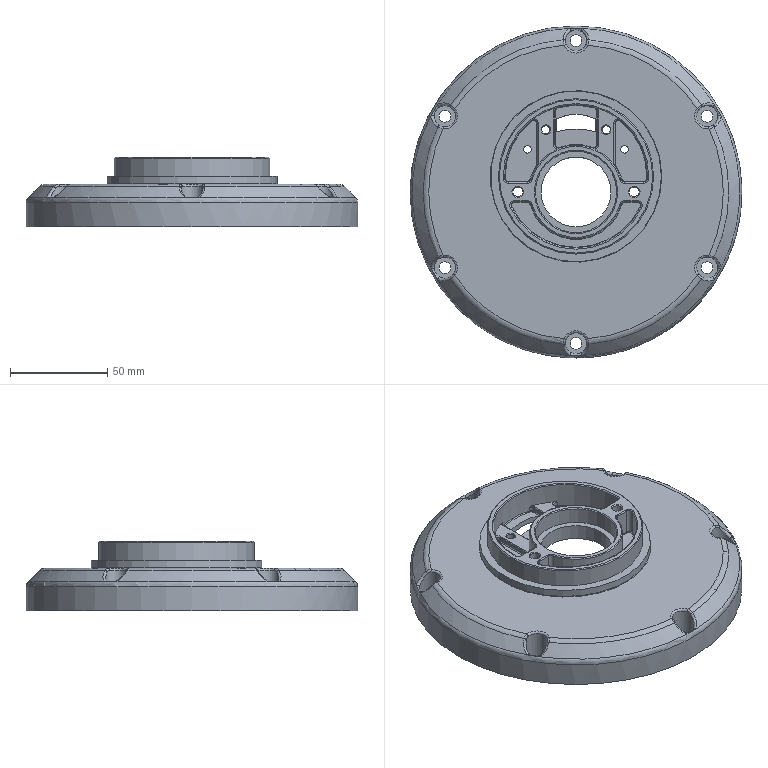NC program | NX | posted with a generic post | part box 171 x 171 x 36 mm
Lines 8896 to 9772 of 127321:
(3D开粗 , TOOL : D6-L25)
N17790 T06 M6
N17792 G54
N17794 G17 G0 G90 X-5.475 Y81.132 S4500 M3
N17796 G43 Z20. H6
N17798 Z-13.83
N17800 G94 G1 Z-14.13 F2500.
N17802 G3 X-4.846 Y79.67 R1.2
N17804 G2 X-3.558 Y78.677 R3.759
N17806 X-2.56 Y76.984 R6.052
N17808 G3 X2.56 Y76.984 R2.755
N17810 G2 X3.545 Y78.661 R6.058
N17812 X4.867 Y79.678 R3.774
N17814 G3 X5.505 Y81.136 R1.2
N17816 G1 Z-13.83
N17818 X-6.033 Y81.749 Z-14.08 F15000.
N17820 Z-14.38 F2500.
N17822 G3 X-5.25 Y80.358 R1.2
N17824 G2 X-3.233 Y78.81 R3.992
N17826 X-2.349 Y77.068 R8.343
N17828 G3 X2.349 Y77.068 R2.527
N17830 G2 X2.709 Y77.901 R96.005
N17832 X4.066 Y79.708 R5.064
N17834 X5.192 Y80.36 R3.692
N17836 G3 X5.953 Y81.755 R1.2
N17838 G1 Z-14.08
N17840 X-6.228 Y82.168 Z-14.33 F15000.
N17842 Z-14.63 F2500.
N17844 G3 X-5.392 Y80.809 R1.2
N17846 G2 X-3.291 Y79.303 R3.983
N17848 G1 X-3.202 Y79.172
N17850 X-2.971 Y78.81
N17852 X-2.955 Y78.782
N17854 X-2.709 Y78.304
N17856 X-2.453 Y77.677
N17858 X-2.437 Y77.624
N17860 X-2.421 Y77.585
N17862 X-2.233 Y77.114
N17864 G3 X2.233 Y77.114 R2.403
N17866 G2 X2.668 Y78.201 R59.523
N17868 X3.714 Y79.793 R5.013
N17870 X5.386 Y80.81 R3.922
N17872 G3 X6.219 Y82.17 R1.2
N17874 G1 Z-14.33
N17876 X-6.346 Y82.495 Z-14.58 F15000.
N17878 Z-14.88 F2500.
N17880 G3 X-5.479 Y81.154 R1.2
N17882 G2 X-3.418 Y79.795 R3.998
N17884 X-2.463 Y77.975 R5.637
N17886 G3 X-2.181 Y77.134 R14.719
N17888 X2.181 Y77.134 R2.346
N17890 G1 X2.232 Y77.263
N17892 X2.463 Y77.973
N17894 G2 X3.418 Y79.795 R5.626
N17896 X5.471 Y81.155 R3.976
N17898 G3 X6.337 Y82.495 R1.2
N17900 G1 Z-14.58
N17902 X-6.409 Y82.764 Z-14.83 F15000.
N17904 Z-15.13 F2500.
N17906 G3 X-5.523 Y81.436 R1.2
N17908 G2 X-3.448 Y80.112 R3.995
N17910 X-2.501 Y78.317 R5.042
N17912 X-2.279 Y77.47 R10.733
N17914 G3 X2.283 Y77.488 R2.34
N17916 G2 X2.677 Y78.81 R8.545
N17918 X3.694 Y80.378 R4.631
N17920 X5.522 Y81.437 R3.974
N17922 G3 X6.407 Y82.765 R1.2
N17924 G1 Z-14.83
N17926 X-6.412 Y83.016 Z-15.08 F15000.
N17928 Z-15.38 F2500.
N17930 G3 X-5.524 Y81.69 R1.2
N17932 G2 X-3.448 Y80.365 R3.982
N17934 G1 X-3.39 Y80.288
N17936 X-3.202 Y80.04
N17938 G2 X-2.362 Y77.947 R5.292
N17940 G1 X-2.344 Y77.825
N17942 X-2.315 Y77.657
N17944 X-2.29 Y77.519
N17946 X-2.279 Y77.47
N17948 G3 X2.283 Y77.488 R2.34
N17950 G1 X2.293 Y77.532
N17952 X2.314 Y77.653
N17954 G2 X2.782 Y79.303 R5.856
N17956 X4.433 Y81.22 R4.368
N17958 X5.516 Y81.69 R3.887
N17960 G3 X6.398 Y83.017 R1.2
N17962 G1 Z-15.08
N17964 X-6.398 Y83.268 Z-15.33 F15000.
N17966 Z-15.63 F2500.
N17968 G3 X-5.513 Y81.941 R1.2
N17970 G2 X-3.694 Y80.884 R3.937
N17972 X-2.436 Y78.463 R4.779
N17974 X-2.33 Y77.788 R4.589
N17976 G3 X-2.29 Y77.519 R2.34
N17978 G1 X-2.279 Y77.47
N17980 G3 X2.283 Y77.488 R2.34
N17982 G1 X2.293 Y77.532
N17984 X2.314 Y77.653
N17986 X2.323 Y77.718
N17988 X2.33 Y77.788
N17990 G2 X2.906 Y79.795 R5.32
N17992 G1 X2.955 Y79.899
N17994 G2 X4.926 Y81.736 R4.272
N17996 X5.495 Y81.942 R3.708
N17998 G3 X6.366 Y83.272 R1.2
N18000 G1 Z-15.33
N18002 X-6.384 Y83.52 Z-15.58 F15000.
N18004 Z-15.88 F2500.
N18006 G3 X-5.501 Y82.193 R1.2
N18008 G2 X-3.694 Y81.144 R3.924
N18010 X-2.6 Y79.303 R4.475
N18012 X-2.337 Y77.89 R5.004
N18014 G1 X-2.333 Y77.82
N18016 X-2.33 Y77.788
N18018 G3 X-2.29 Y77.519 R2.34
N18020 G1 X-2.279 Y77.47
N18022 G3 X2.283 Y77.488 R2.34
N18024 G1 X2.293 Y77.532
N18026 X2.314 Y77.653
N18028 X2.323 Y77.718
N18030 X2.337 Y77.89
N18032 G2 X2.784 Y79.795 R5.282
N18034 G1 X2.955 Y80.157
N18036 X3.154 Y80.471
N18038 G2 X4.636 Y81.842 R3.941
N18040 G1 X4.716 Y81.884
N18042 G2 X5.497 Y82.193 R3.764
N18044 G3 X6.372 Y83.522 R1.2
N18046 G1 Z-15.58
N18048 X-6.344 Y83.774 Z-15.83 F15000.
N18050 Z-16.13 F2500.
N18052 G3 X-5.466 Y82.446 R1.2
N18054 G2 X-4.11 Y81.775 R3.835
N18056 X-2.671 Y79.795 R4.362
N18058 X-2.34 Y77.98 R5.395
N18060 G1 X-2.333 Y77.82
N18062 X-2.33 Y77.788
N18064 X-2.322 Y77.711
N18066 X-2.29 Y77.519
N18068 X-2.279 Y77.47
N18070 G3 X2.283 Y77.488 R2.34
N18072 G1 X2.293 Y77.532
N18074 X2.314 Y77.653
N18076 X2.323 Y77.718
N18078 G3 X2.34 Y77.98 R2.34
N18080 G2 X2.73 Y79.95 R5.395
N18082 X4.05 Y81.729 R4.377
N18084 X5.466 Y82.446 R3.844
N18086 G3 X6.345 Y83.774 R1.2
N18088 G1 Z-15.83
N18090 X-6.319 Y84.026 Z-16.08 F15000.
N18092 Z-16.38 F2500.
N18094 G3 X-5.438 Y82.697 R1.2
N18096 G2 X-3.202 Y81.118 R3.928
N18098 G1 X-2.993 Y80.78
N18100 X-2.955 Y80.721
N18102 X-2.745 Y80.288
N18104 X-2.709 Y80.206
N18106 X-2.607 Y79.904
N18108 G2 X-2.336 Y78.317 R5.125
N18110 G1 X-2.343 Y78.253
N18112 X-2.339 Y78.163
N18114 Y78.071
N18116 G3 X-2.333 Y77.82 R2.34
N18118 G1 X-2.33 Y77.788
N18120 X-2.321 Y77.705
N18122 X-2.29 Y77.519
N18124 X-2.279 Y77.47
N18126 G3 X2.283 Y77.488 R2.34
N18128 G1 X2.293 Y77.532
N18130 X2.314 Y77.653
N18132 X2.323 Y77.718
N18134 G3 X2.339 Y78.071 R2.34
N18136 G2 X2.441 Y79.303 R5.682
N18138 X3.448 Y81.439 R4.76
N18140 X5.432 Y82.697 R3.907
N18142 G3 X6.312 Y84.026 R1.2
N18144 G1 Z-16.08
N18146 X-6.256 Y84.282 Z-16.33 F15000.
N18148 Z-16.63 F2500.
N18150 G3 X-5.379 Y82.952 R1.2
N18152 G2 X-3.384 Y81.659 R3.854
N18154 X-2.416 Y79.549 R4.658
N18156 X-2.334 Y78.162 R5.651
N18158 G3 X-2.337 Y77.89 R2.34
N18160 G1 X-2.333 Y77.82
N18162 X-2.33 Y77.788
N18164 G3 X-2.29 Y77.519 R2.34
N18166 G1 X-2.279 Y77.47
N18168 G3 X2.266 Y77.416 R2.34
N18170 G1 X2.283 Y77.488
N18172 X2.293 Y77.532
N18174 X2.314 Y77.653
N18176 X2.325 Y77.738
N18178 X2.333 Y77.818
N18180 X2.338 Y77.899
N18182 G3 X2.335 Y78.152 R2.34
N18184 G2 X2.69 Y80.49 R5.29
N18186 X3.943 Y82.211 R4.254
N18188 X5.38 Y82.952 R3.828
N18190 G3 X6.255 Y84.282 R1.2
N18192 G1 Z-16.33
N18194 X-6.245 Y84.533 Z-16.58 F15000.
N18196 Z-16.88 F2500.
N18198 G3 X-5.36 Y83.206 R1.2
N18200 G2 X-2.955 Y81.373 R3.925
N18202 X-2.299 Y79.042 R4.937
N18204 X-2.326 Y78.253 R5.852
N18206 G3 X-2.333 Y77.82 R2.34
N18208 G1 X-2.33 Y77.788
N18210 G3 X-2.29 Y77.519 R2.34
N18212 G1 X-2.279 Y77.47
N18214 X-2.272 Y77.44
N18216 G3 X2.283 Y77.488 R2.34
N18218 G1 X2.293 Y77.532
N18220 X2.314 Y77.653
N18222 X2.325 Y77.738
N18224 X2.335 Y77.843
N18226 G3 X2.335 Y78.152 R2.34
N18228 G1 X2.333 Y78.183
N18230 X2.325 Y78.264
N18232 G2 X2.709 Y80.902 R5.234
N18234 X4.433 Y82.841 R4.181
N18236 X5.335 Y83.208 R3.847
N18238 G3 X6.216 Y84.535 R1.2
N18240 G1 Z-16.58
N18242 X-6.158 Y84.791 Z-16.83 F15000.
N18244 Z-17.13 F2500.
N18246 G3 X-5.279 Y83.46 R1.2
N18248 G2 X-2.706 Y81.273 R3.924
N18250 X-2.294 Y78.532 R5.128
N18252 G1 X-2.314 Y78.345
N18254 G3 X-2.336 Y77.867 R2.34
N18256 G1 X-2.333 Y77.82
N18258 X-2.33 Y77.788
N18260 G3 X-2.29 Y77.519 R2.34
N18262 G1 X-2.278 Y77.463
N18264 G3 X2.283 Y77.488 R2.34
N18266 G1 X2.293 Y77.532
N18268 X2.314 Y77.653
N18270 X2.323 Y77.718
N18272 G3 X2.335 Y78.152 R2.34
N18274 G1 X2.333 Y78.183
N18276 X2.314 Y78.345
N18278 G2 X2.51 Y80.78 R5.325
N18280 X4.926 Y83.358 R4.062
N18282 X5.24 Y83.463 R3.593
N18284 G3 X6.1 Y84.797 R1.2
N18286 G1 Z-16.83
N18288 X-6.065 Y85.047 Z-17.08 F15000.
N18290 Z-17.38 F2500.
N18292 G3 X-5.189 Y83.715 R1.2
N18294 G2 X-2.528 Y81.273 R3.915
N18296 X-2.271 Y78.624 R5.144
N18298 G1 X-2.318 Y78.317
N18300 G3 X-2.337 Y77.89 R2.34
N18302 G1 X-2.333 Y77.82
N18304 X-2.33 Y77.788
N18306 G3 X-2.29 Y77.519 R2.34
N18308 G1 X-2.279 Y77.47
N18310 G3 X2.283 Y77.488 R2.34
N18312 G1 X2.293 Y77.532
N18314 X2.314 Y77.653
N18316 X2.323 Y77.718
N18318 X2.338 Y77.899
N18320 G3 X2.335 Y78.152 R2.34
N18322 G1 X2.333 Y78.183
N18324 G3 X2.299 Y78.436 R2.34
N18326 G2 X2.264 Y80.288 R5.517
N18328 X3.065 Y82.258 R4.438
N18330 X5.17 Y83.716 R3.843
N18332 G3 X6.042 Y85.049 R1.2
N18334 G1 Z-17.08
N18336 X-5.966 Y85.306 Z-17.33 F15000.
N18338 Z-17.63 F2500.
N18340 G3 X-5.092 Y83.973 R1.2
N18342 G2 X-2.542 Y81.765 R3.882
N18344 X-2.207 Y78.915 R5.025
N18346 G1 X-2.279 Y78.529
N18348 X-2.307 Y78.393
N18350 X-2.318 Y78.317
N18352 G3 X-2.337 Y77.89 R2.34
N18354 G1 X-2.333 Y77.82
N18356 X-2.33 Y77.788
N18358 G3 X-2.29 Y77.519 R2.34
N18360 G1 X-2.279 Y77.47
N18362 G3 X2.283 Y77.488 R2.34
N18364 G1 X2.293 Y77.532
N18366 X2.301 Y77.575
N18368 X2.314 Y77.653
N18370 X2.323 Y77.718
N18372 X2.327 Y77.75
N18374 X2.338 Y77.899
N18376 G3 X2.335 Y78.152 R2.34
N18378 G1 X2.333 Y78.183
N18380 G3 X2.28 Y78.529 R2.34
N18382 G2 X2.229 Y80.78 R5.431
N18384 X3.448 Y83.057 R4.27
N18386 X5.047 Y83.976 R3.724
N18388 G3 X5.912 Y85.311 R1.2
N18390 G1 Z-17.33
N18392 X-5.828 Y85.566 Z-17.58 F15000.
N18394 Z-17.88 F2500.
N18396 G3 X-4.961 Y84.231 R1.2
N18398 G2 X-2.861 Y82.75 R3.807
N18400 X-2.089 Y80.65 R4.204
N18402 G1 X-2.078 Y80.514
N18404 G2 X-2.255 Y78.623 R5.42
N18406 G3 X-2.307 Y78.393 R2.34
N18408 G1 X-2.318 Y78.317
N18410 G3 X-2.337 Y77.89 R2.34
N18412 G1 X-2.333 Y77.82
N18414 X-2.33 Y77.788
N18416 G3 X-2.29 Y77.519 R2.34
N18418 G1 X-2.279 Y77.47
N18420 G3 X2.283 Y77.488 R2.34
N18422 G1 X2.293 Y77.532
N18424 X2.314 Y77.653
N18426 X2.323 Y77.718
N18428 G3 X2.335 Y78.152 R2.34
N18430 G1 X2.333 Y78.183
N18432 G3 X2.256 Y78.621 R2.34
N18434 G2 X2.217 Y81.383 R5.381
N18436 X3.94 Y83.781 R4.077
N18438 X4.932 Y84.232 R3.652
N18440 G3 X5.79 Y85.57 R1.2
N18442 G1 Z-17.58
N18444 X-5.729 Y85.823 Z-17.83 F15000.
N18446 Z-18.13 F2500.
N18448 G3 X-4.86 Y84.487 R1.2
N18450 G2 X-2.145 Y81.765 R3.876
N18452 G1 X-2.03 Y81.273
N18454 G2 X-2.134 Y79.045 R5.404
N18456 G1 X-2.179 Y78.904
N18458 X-2.229 Y78.713
N18460 G3 X-2.307 Y78.393 R2.34
N18462 G1 X-2.318 Y78.317
N18464 G3 X-2.337 Y77.89 R2.34
N18466 G1 X-2.333 Y77.82
N18468 X-2.33 Y77.788
N18470 G3 X-2.29 Y77.519 R2.34
N18472 G1 X-2.279 Y77.47
N18474 G3 X2.283 Y77.488 R2.34
N18476 G1 X2.293 Y77.532
N18478 X2.314 Y77.653
N18480 X2.323 Y77.718
N18482 G3 X2.335 Y78.152 R2.34
N18484 G1 X2.333 Y78.183
N18486 G3 X2.232 Y78.703 R2.34
N18488 G2 X2.03 Y81.273 R5.484
N18490 X3.448 Y83.767 R4.13
N18492 X4.837 Y84.489 R3.803
N18494 G3 X5.702 Y85.825 R1.2
N18496 G1 Z-17.83
N18498 X-5.583 Y86.084 Z-18.08 F15000.
N18500 Z-18.38 F2500.
N18502 G3 X-4.716 Y84.747 R1.2
N18504 G2 X-1.97 Y81.824 R3.857
N18506 X-2.132 Y78.996 R5.26
N18508 G1 X-2.134 Y78.985
N18510 X-2.167 Y78.9
N18512 X-2.197 Y78.805
N18514 G3 X-2.307 Y78.393 R2.34
N18516 G1 X-2.318 Y78.317
N18518 G3 X-2.333 Y77.82 R2.34
N18520 G1 X-2.33 Y77.788
N18522 G3 X-2.29 Y77.519 R2.34
N18524 G1 X-2.279 Y77.47
N18526 G3 X2.283 Y77.488 R2.34
N18528 G1 X2.293 Y77.532
N18530 X2.314 Y77.653
N18532 X2.323 Y77.718
N18534 G3 X2.335 Y78.152 R2.34
N18536 G1 X2.333 Y78.183
N18538 G3 X2.232 Y78.703 R2.34
N18540 G1 X2.221 Y78.736
N18542 X2.197 Y78.805
N18544 G2 X1.874 Y81.273 R5.553
N18546 X2.955 Y83.697 R4.229
N18548 X4.703 Y84.748 R3.826
N18550 G3 X5.567 Y86.085 R1.2
N18552 G1 Z-18.08
N18554 X-5.412 Y86.345 Z-18.33 F15000.
N18556 Z-18.63 F2500.
N18558 G3 X-4.55 Y85.006 R1.2
N18560 G2 X-1.869 Y82.258 R3.832
N18562 G1 X-1.77 Y81.765
N18564 G2 X-2.049 Y79.19 R5.302
N18566 G1 X-2.091 Y79.092
N18568 X-2.161 Y78.898
N18570 G3 X-2.307 Y78.393 R2.34
N18572 G1 X-2.318 Y78.317
N18574 G3 X-2.337 Y77.89 R2.34
N18576 G1 X-2.333 Y77.82
N18578 X-2.33 Y77.788
N18580 G3 X-2.29 Y77.519 R2.34
N18582 G1 X-2.279 Y77.47
N18584 G3 X2.283 Y77.488 R2.34
N18586 G1 X2.293 Y77.532
N18588 X2.314 Y77.653
N18590 X2.323 Y77.718
N18592 G3 X2.335 Y78.152 R2.34
N18594 G1 X2.333 Y78.183
N18596 G3 X2.251 Y78.638 R2.34
N18598 G1 X2.232 Y78.703
N18600 X2.221 Y78.736
N18602 X2.191 Y78.82
N18604 X2.161 Y78.898
N18606 G2 X1.87 Y79.795 R6.981
N18608 X1.97 Y82.579 R4.89
N18610 X4.545 Y85.006 R3.817
N18612 G3 X5.406 Y86.346 R1.2
N18614 G1 Z-18.33
N18616 X-5.233 Y86.607 Z-18.58 F15000.
N18618 Z-18.88 F2500.
N18620 G3 X-4.374 Y85.266 R1.2
N18622 G2 X-1.649 Y82.258 R3.826
N18624 X-1.97 Y79.339 R5.327
N18626 G1 X-1.985 Y79.303
N18628 X-2.039 Y79.186
N18630 X-2.134 Y78.959
N18632 G3 X-2.307 Y78.393 R2.34
N18634 G1 X-2.318 Y78.317
N18636 G3 X-2.333 Y77.82 R2.34
N18638 G1 X-2.33 Y77.788
N18640 G3 X-2.29 Y77.518 R2.34
N18642 G1 X-2.279 Y77.47
N18644 G3 X2.283 Y77.488 R2.34
N18646 G1 X2.293 Y77.532
N18648 X2.314 Y77.653
N18650 X2.323 Y77.718
N18652 X2.333 Y77.816
N18654 G3 X2.335 Y78.152 R2.34
N18656 G1 X2.333 Y78.183
N18658 G3 X2.232 Y78.703 R2.34
N18660 G1 X2.221 Y78.736
N18662 G3 X2.12 Y78.991 R2.34
N18664 G2 X1.809 Y79.795 R8.055
N18666 X1.648 Y82.258 R5.191
N18668 X4.373 Y85.266 R3.825
N18670 G3 X5.232 Y86.607 R1.2
N18672 G1 Z-18.58
N18674 X-5.009 Y86.87 Z-18.83 F15000.
N18676 Z-19.13 F2500.
N18678 G3 X-4.158 Y85.525 R1.2
N18680 G2 X-1.477 Y82.527 R3.788
N18682 X-1.609 Y80.242 R5.076
N18684 X-2.085 Y79.062 R6.477
N18686 G3 X-2.307 Y78.393 R2.34
N18688 G1 X-2.318 Y78.317
N18690 G3 X-2.337 Y77.89 R2.34
N18692 G1 X-2.333 Y77.82
N18694 X-2.33 Y77.788
N18696 G3 X-2.29 Y77.518 R2.34
N18698 G1 X-2.279 Y77.47
N18700 G3 X2.283 Y77.488 R2.34
N18702 G1 X2.293 Y77.532
N18704 X2.314 Y77.653
N18706 X2.323 Y77.722
N18708 G3 X2.335 Y78.152 R2.34
N18710 G1 X2.333 Y78.183
N18712 G3 X2.232 Y78.703 R2.34
N18714 G1 X2.221 Y78.738
N18716 X2.191 Y78.82
N18718 G3 X2.074 Y79.084 R2.34
N18720 G2 X1.597 Y80.288 R6.965
N18722 X1.522 Y82.75 R4.849
N18724 X4.156 Y85.525 R3.787
N18726 G3 X5.007 Y86.87 R1.2
N18728 G1 Z-18.83
N18730 X-4.792 Y87.133 Z-19.08 F15000.
N18732 Z-19.38 F2500.
N18734 G3 X-3.943 Y85.786 R1.2
N18736 G2 X-1.21 Y82.258 R3.796
N18738 X-1.735 Y79.728 R5.463
N18740 X-2.022 Y79.178 R8.409
N18742 G1 X-2.068 Y79.095
N18744 X-2.085 Y79.062
N18746 G3 X-2.307 Y78.393 R2.34
N18748 G1 X-2.318 Y78.317
N18750 G3 X-2.336 Y77.867 R2.34
N18752 G1 X-2.333 Y77.82
N18754 X-2.33 Y77.788
N18756 G3 X-2.29 Y77.518 R2.34
N18758 G1 X-2.279 Y77.47
N18760 G3 X2.283 Y77.488 R2.34
N18762 G1 X2.293 Y77.532
N18764 X2.314 Y77.653
N18766 X2.323 Y77.722
N18768 X2.333 Y77.816
N18770 X2.338 Y77.899
N18772 G3 X2.335 Y78.152 R2.34
N18774 G1 X2.331 Y78.204
N18776 X2.313 Y78.356
N18778 X2.299 Y78.437
N18780 X2.277 Y78.54
N18782 X2.251 Y78.638
N18784 X2.232 Y78.703
N18786 X2.221 Y78.738
N18788 X2.191 Y78.82
N18790 X2.133 Y78.962
N18792 X2.12 Y78.991
N18794 G3 X2.022 Y79.178 R2.34
N18796 G2 X1.22 Y81.611 R5.957
N18798 X2.214 Y84.721 R4.085
N18800 X3.944 Y85.786 R3.814
N18802 G3 X4.793 Y87.133 R1.2
N18804 G1 Z-19.08
N18806 X-4.529 Y87.398 Z-19.33 F15000.
N18808 Z-19.63 F2500.
N18810 G3 X-3.686 Y86.048 R1.2
N18812 G2 X-0.985 Y82.515 R3.773
N18814 X-1.423 Y80.291 R5.27
N18816 X-1.964 Y79.273 R7.469
N18818 G3 X-2.068 Y79.095 R2.34
N18820 G1 X-2.085 Y79.062
N18822 G3 X-2.307 Y78.393 R2.34
N18824 G1 X-2.318 Y78.317
N18826 G3 X-2.337 Y77.89 R2.34
N18828 G1 X-2.333 Y77.82
N18830 X-2.33 Y77.788
N18832 G3 X-2.29 Y77.518 R2.34
N18834 G1 X-2.279 Y77.47
N18836 G3 X2.283 Y77.488 R2.34
N18838 G1 X2.293 Y77.532
N18840 X2.314 Y77.653
N18842 X2.323 Y77.718
N18844 X2.333 Y77.816
N18846 X2.338 Y77.899
N18848 G3 X2.335 Y78.152 R2.34
N18850 G1 X2.333 Y78.183
N18852 G3 X2.277 Y78.54 R2.34
N18854 G1 X2.251 Y78.638
N18856 X2.232 Y78.703
N18858 X2.221 Y78.736
N18860 X2.191 Y78.82
N18862 G3 X1.964 Y79.272 R2.34
N18864 G2 X1.325 Y80.534 R7.072
N18866 X0.985 Y82.549 R5.201
N18868 X3.682 Y86.048 R3.771
N18870 G3 X4.524 Y87.398 R1.2
N18872 G1 Z-19.33
N18874 X-4.251 Y87.662 Z-19.58 F15000.
N18876 Z-19.88 F2500.
N18878 G3 X-3.413 Y86.31 R1.2
N18880 G2 X-0.749 Y82.258 R3.772
N18882 G1 X-0.82 Y81.765
N18884 G2 X-1.806 Y79.506 R6.112
N18886 G1 X-1.835 Y79.469
N18888 X-1.899 Y79.367
N18890 G3 X-2.068 Y79.095 R2.34
N18892 G1 X-2.085 Y79.062
N18894 G3 X-2.307 Y78.393 R2.34
N18896 G1 X-2.318 Y78.317
N18898 G3 X-2.337 Y77.89 R2.34
N18900 G1 X-2.333 Y77.82
N18902 X-2.33 Y77.788
N18904 G3 X-2.29 Y77.518 R2.34
N18906 G1 X-2.279 Y77.47
N18908 G3 X2.275 Y77.453 R2.34
N18910 G1 X2.283 Y77.488
N18912 X2.293 Y77.532
N18914 X2.314 Y77.653
N18916 X2.325 Y77.734
N18918 X2.338 Y77.899
N18920 G3 X2.335 Y78.152 R2.34
N18922 G1 X2.333 Y78.183
N18924 G3 X2.277 Y78.54 R2.34
N18926 G1 X2.251 Y78.638
N18928 X2.232 Y78.703
N18930 X2.221 Y78.736
N18932 X2.191 Y78.82
N18934 G3 X1.899 Y79.367 R2.34
N18936 G2 X1.22 Y80.534 R7.37
N18938 X0.719 Y82.75 R5.392
N18940 X3.41 Y86.31 R3.775
N18942 G3 X4.249 Y87.662 R1.2
N18944 G1 Z-19.58
N18946 X-3.943 Y87.926 Z-19.83 F15000.
N18948 Z-20.13 F2500.
N18950 G3 X-3.107 Y86.571 R1.2
N18952 G2 X-0.84 Y84.721 R3.83
N18954 X-0.64 Y81.639 R4.134
N18956 X-1.827 Y79.462 R6.884
N18958 G3 X-2.068 Y79.095 R2.34
N18960 G1 X-2.085 Y79.062
N18962 G3 X-2.307 Y78.393 R2.34
N18964 G1 X-2.318 Y78.317
N18966 G3 X-2.333 Y77.82 R2.34
N18968 G1 X-2.33 Y77.788
N18970 G3 X-2.29 Y77.518 R2.34
N18972 G1 X-2.279 Y77.47
N18974 G3 X2.283 Y77.488 R2.34
N18976 G1 X2.293 Y77.532
N18978 X2.314 Y77.653
N18980 X2.323 Y77.718
N18982 G3 X2.335 Y78.152 R2.34
N18984 G1 X2.333 Y78.183
N18986 G3 X2.232 Y78.704 R2.34
N18988 G1 X2.221 Y78.736
N18990 G3 X1.827 Y79.462 R2.34
N18992 G2 X0.638 Y81.642 R6.843
N18994 X0.839 Y84.721 R4.137
N18996 X3.106 Y86.571 R3.829
N18998 G3 X3.942 Y87.926 R1.2
N19000 G1 Z-19.83
N19002 X-3.593 Y88.19 Z-20.08 F15000.
N19004 Z-20.38 F2500.
N19006 G3 X-2.75 Y86.833 R1.2
N19008 G2 X-1.478 Y86.199 R4.062
N19010 X-0.268 Y82.063 R3.771
N19012 X-1.301 Y80.11 R6.821
N19014 G1 X-1.478 Y79.876
N19016 X-1.543 Y79.795
N19018 X-1.57 Y79.763
N19020 X-1.642 Y79.684
N19022 X-1.664 Y79.66
N19024 X-1.746 Y79.557
N19026 G3 X-2.068 Y79.095 R2.34
N19028 G1 X-2.085 Y79.062
N19030 G3 X-2.307 Y78.393 R2.34
N19032 G1 X-2.318 Y78.317
N19034 G3 X-2.333 Y77.82 R2.34
N19036 G1 X-2.33 Y77.788
N19038 G3 X-2.29 Y77.518 R2.34
N19040 G1 X-2.279 Y77.47
N19042 G3 X2.283 Y77.488 R2.34
N19044 G1 X2.293 Y77.532
N19046 X2.314 Y77.653
N19048 X2.323 Y77.718
N19050 X2.333 Y77.816
N19052 X2.338 Y77.899
N19054 G3 X2.335 Y78.152 R2.34
N19056 G1 X2.333 Y78.183
N19058 G3 X2.277 Y78.54 R2.34
N19060 G1 X2.251 Y78.638
N19062 X2.232 Y78.704
N19064 X2.221 Y78.736
N19066 X2.191 Y78.82
N19068 G3 X1.747 Y79.557 R2.34
N19070 G2 X0.436 Y81.602 R7.492
N19072 X0.101 Y83.67 R4.298
N19074 X2.713 Y86.834 R3.608
N19076 G3 X3.572 Y88.17 R1.2
N19078 G1 Z-20.08
N19080 X-3.119 Y88.452 Z-20.33 F15000.
N19082 Z-20.63 F2500.
N19084 G3 X-2.24 Y87.099 R1.2
N19086 G2 X-1.191 Y86.691 R5.01
N19088 X0. Y85.461 R2.735
N19090 X1.97 Y87.031 R3.381
N19092 X2.23 Y87.099 R6.01
N19094 G3 X3.14 Y88.445 R1.2
N19096 G1 Z-20.33
N19098 G0 Z20.
N19100 X-2.13 Y77.375
N19102 Z-19.38
N19104 G3 X-2.13 Y77.375 Z-19.88 I2.188 J0.641
N19106 X-2.13 Y77.375 Z-20.381 I2.188 J0.641
N19108 X2.251 Y78.639 Z-20.63 R2.28
N19110 G1 X2.248 Y78.65
N19112 X2.245 Y78.659
N19114 X2.232 Y78.704
N19116 X2.221 Y78.736
N19118 G3 X1.657 Y79.652 R2.34
N19120 G2 X0.384 Y81.273 R8.531
N19122 X0. Y82.034 R5.24
N19124 X-1.296 Y80.041 R7.204
N19126 G1 X-1.657 Y79.653
N19128 G3 X-2.068 Y79.095 R2.34
N19130 G1 X-2.085 Y79.062
N19132 G3 X-2.307 Y78.393 R2.34
N19134 G1 X-2.318 Y78.317
N19136 G3 X-2.333 Y77.82 R2.34
N19138 G1 X-2.33 Y77.788
N19140 G3 X-2.301 Y77.576 R2.34
N19142 G1 X-2.271 Y77.434
N19144 G3 X2.283 Y77.488 R2.34
N19146 G1 X2.294 Y77.54
N19148 X2.3 Y77.582
N19150 X2.304 Y77.592
N19152 X2.314 Y77.653
N19154 X2.323 Y77.718
N19156 G3 X2.335 Y78.152 R2.34
N19158 G1 X2.333 Y78.183
N19160 G3 X2.248 Y78.65 R2.34
N19162 G1 X2.245 Y78.659
N19164 X2.232 Y78.704
N19166 X2.221 Y78.736
N19168 G3 X2.059 Y79.112 R2.34
N19170 X0.433 Y79.598 R1.2
N19172 G1 Z-20.33
N19174 X-2.13 Y77.375 Z-19.63 F15000.
N19176 G3 X-2.13 Y77.375 Z-20.13 I2.188 J0.641 F2500.
N19178 X-2.13 Y77.375 Z-20.631 I2.188 J0.641
N19180 X2.251 Y78.639 Z-20.88 R2.28
N19182 G1 X2.248 Y78.65
N19184 X2.232 Y78.704
N19186 X2.221 Y78.736
N19188 G3 X1.556 Y79.748 R2.34
N19190 G2 X0.525 Y80.809 R10.541
N19192 G3 X-0.521 Y80.812 R3.78
N19194 G2 X-1.556 Y79.748 R11.179
N19196 G3 X-2.068 Y79.095 R2.34
N19198 G1 X-2.085 Y79.062
N19200 G3 X-2.307 Y78.393 R2.34
N19202 G1 X-2.318 Y78.317
N19204 G3 X-2.333 Y77.82 R2.34
N19206 G1 X-2.33 Y77.788
N19208 G3 X-2.301 Y77.576 R2.34
N19210 G1 X-2.271 Y77.434
N19212 G3 X2.283 Y77.488 R2.34
N19214 G1 X2.294 Y77.54
N19216 X2.3 Y77.582
N19218 X2.304 Y77.592
N19220 X2.314 Y77.653
N19222 X2.323 Y77.718
N19224 G3 X2.335 Y78.152 R2.34
N19226 G1 X2.333 Y78.183
N19228 G3 X2.248 Y78.65 R2.34
N19230 G1 X2.232 Y78.704
N19232 X2.221 Y78.736
N19234 G3 X2.059 Y79.112 R2.34
N19236 X0.433 Y79.598 R1.2
N19238 G1 Z-20.58
N19240 X-2.13 Y77.375 Z-19.88 F15000.
N19242 G3 X-2.13 Y77.375 Z-20.38 I2.188 J0.641 F2500.
N19244 X-2.13 Y77.375 Z-20.881 I2.188 J0.641
N19246 X2.251 Y78.639 Z-21.13 R2.28
N19248 G1 X2.248 Y78.65
N19250 X2.232 Y78.704
N19252 X2.221 Y78.736
N19254 G3 X1.441 Y79.843 R2.34
N19256 G2 X0.67 Y80.495 R17.552
N19258 G3 X-0.672 Y80.495 R2.773
N19260 G2 X-1.441 Y79.844 R17.849
N19262 G3 X-2.068 Y79.095 R2.34
N19264 G1 X-2.085 Y79.062
N19266 G3 X-2.307 Y78.393 R2.34
N19268 G1 X-2.318 Y78.317
N19270 G3 X-2.333 Y77.82 R2.34
N19272 G1 X-2.33 Y77.788
N19274 G3 X-2.301 Y77.576 R2.34
N19276 G1 X-2.271 Y77.434
N19278 G3 X2.283 Y77.488 R2.34
N19280 G1 X2.294 Y77.54
N19282 X2.3 Y77.582
N19284 X2.304 Y77.592
N19286 X2.314 Y77.653
N19288 X2.323 Y77.718
N19290 X2.327 Y77.757
N19292 G3 X2.335 Y78.152 R2.34
N19294 G1 X2.333 Y78.183
N19296 G3 X2.248 Y78.65 R2.34
N19298 G1 X2.232 Y78.704
N19300 X2.221 Y78.736
N19302 G3 X2.059 Y79.112 R2.34
N19304 X0.433 Y79.598 R1.2
N19306 G1 Z-20.83
N19308 X-2.13 Y77.375 Z-20.13 F15000.
N19310 G3 X-2.13 Y77.375 Z-20.63 I2.188 J0.641 F2500.
N19312 X-2.13 Y77.375 Z-21.131 I2.188 J0.641
N19314 X2.251 Y78.639 Z-21.38 R2.28
N19316 G1 X2.248 Y78.65
N19318 X2.232 Y78.704
N19320 X2.221 Y78.735
N19322 G3 X1.309 Y79.939 R2.34
N19324 G1 X1.231 Y79.994
N19326 X0.793 Y80.288
N19328 X0.739 Y80.315
N19330 G3 X-0.739 Y80.315 R2.365
N19332 G1 X-0.793 Y80.288
N19334 X-1.231 Y79.996
N19336 X-1.309 Y79.939
N19338 G3 X-2.068 Y79.095 R2.34
N19340 G1 X-2.085 Y79.062
N19342 G3 X-2.307 Y78.393 R2.34
N19344 G1 X-2.318 Y78.317
N19346 G3 X-2.333 Y77.819 R2.34
N19348 G1 X-2.33 Y77.788
N19350 X-2.313 Y77.648
N19352 X-2.301 Y77.576
N19354 X-2.271 Y77.434
N19356 G3 X2.283 Y77.488 R2.34
N19358 G1 X2.294 Y77.54
N19360 X2.3 Y77.583
N19362 X2.304 Y77.592
N19364 X2.314 Y77.653
N19366 X2.323 Y77.718
N19368 G3 X2.335 Y78.152 R2.34
N19370 G1 X2.333 Y78.183
N19372 G3 X2.248 Y78.65 R2.34
N19374 G1 X2.232 Y78.704
N19376 X2.221 Y78.735
N19378 G3 X2.059 Y79.112 R2.34
N19380 X0.433 Y79.598 R1.2
N19382 G1 Z-21.08
N19384 X-2.13 Y77.375 Z-20.38 F15000.
N19386 G3 X-2.13 Y77.375 Z-20.88 I2.188 J0.641 F2500.
N19388 X-2.13 Y77.375 Z-21.381 I2.188 J0.641
N19390 X2.251 Y78.639 Z-21.63 R2.28
N19392 G1 X2.248 Y78.65
N19394 X2.232 Y78.704
N19396 X2.221 Y78.735
N19398 G3 X1.144 Y80.041 R2.34
N19400 X0.56 Y80.288 R1.907
N19402 X-0.56 Y80.288 R2.393
N19404 X-1.153 Y80.036 R1.922
N19406 X-2.068 Y79.095 R2.34
N19408 G1 X-2.085 Y79.062
N19410 G3 X-2.307 Y78.393 R2.34
N19412 G1 X-2.318 Y78.317
N19414 G3 X-2.333 Y77.819 R2.34
N19416 G1 X-2.33 Y77.788
N19418 X-2.313 Y77.648
N19420 X-2.301 Y77.576
N19422 X-2.271 Y77.434
N19424 G3 X2.283 Y77.488 R2.34
N19426 G1 X2.294 Y77.54
N19428 X2.3 Y77.583
N19430 X2.304 Y77.592
N19432 X2.314 Y77.653
N19434 X2.323 Y77.718
N19436 G3 X2.335 Y78.152 R2.34
N19438 G1 X2.333 Y78.183
N19440 G3 X2.248 Y78.65 R2.34
N19442 G1 X2.232 Y78.704
N19444 X2.221 Y78.735
N19446 G3 X2.059 Y79.112 R2.34
N19448 X0.433 Y79.598 R1.2
N19450 G1 Z-21.33
N19452 X-2.13 Y77.375 Z-20.63 F15000.
N19454 G3 X-2.13 Y77.375 Z-21.13 I2.188 J0.641 F2500.
N19456 X-2.13 Y77.375 Z-21.631 I2.188 J0.641
N19458 X2.251 Y78.639 Z-21.88 R2.28
N19460 G1 X2.248 Y78.65
N19462 X2.232 Y78.704
N19464 X2.214 Y78.757
N19466 G3 X-2.068 Y79.095 R2.34
N19468 G1 X-2.085 Y79.062
N19470 G3 X-2.307 Y78.393 R2.34
N19472 G1 X-2.318 Y78.317
N19474 G3 X-2.333 Y77.819 R2.34
N19476 G1 X-2.33 Y77.788
N19478 X-2.313 Y77.648
N19480 X-2.301 Y77.576
N19482 X-2.271 Y77.434
N19484 G3 X2.283 Y77.488 R2.34
N19486 G1 X2.294 Y77.54
N19488 X2.3 Y77.583
N19490 X2.304 Y77.592
N19492 X2.314 Y77.653
N19494 X2.323 Y77.717
N19496 G3 X2.335 Y78.152 R2.34
N19498 G1 X2.333 Y78.183
N19500 G3 X2.248 Y78.65 R2.34
N19502 G1 X2.232 Y78.704
N19504 X2.214 Y78.757
N19506 G3 X2.059 Y79.112 R2.34
N19508 X0.433 Y79.598 R1.2
N19510 G1 Z-21.58
N19512 X-2.13 Y77.375 Z-20.88 F15000.
N19514 G3 X-2.13 Y77.375 Z-21.38 I2.188 J0.641 F2500.
N19516 X-2.13 Y77.375 Z-21.881 I2.188 J0.641
N19518 X2.251 Y78.639 Z-22.13 R2.28
N19520 G1 X2.248 Y78.65
N19522 X2.247 Y78.652
N19524 X2.232 Y78.704
N19526 X2.214 Y78.757
N19528 G3 X0.489 Y80.288 R2.34
N19530 X-2.068 Y79.095 R2.34
N19532 G1 X-2.085 Y79.062
N19534 G3 X-2.307 Y78.393 R2.34
N19536 G1 X-2.318 Y78.317